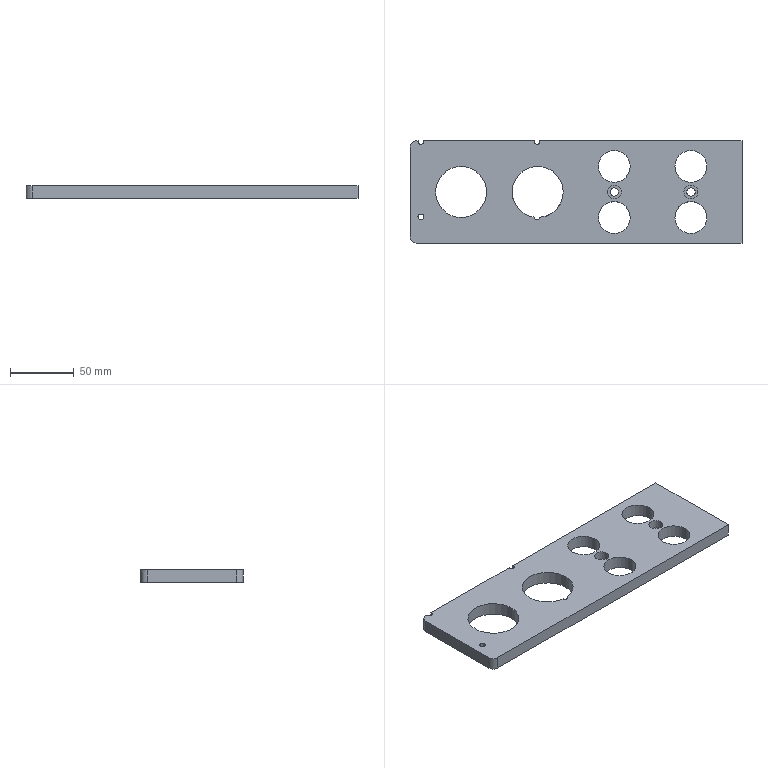Part | SolidWorks | features HoleWzd 3, ICE 2, Extrusion 1, Fillet 1 | 1 solid | 64 faces | box 260 x 80 x 10 mm | volume 160429 mm3 | cylinder 46 | plane 14 | cone 4 | commonest cylinder face diameters 8 x10 4.5 x9 25 x8 40 x5 4.2 x4 6.6 x4